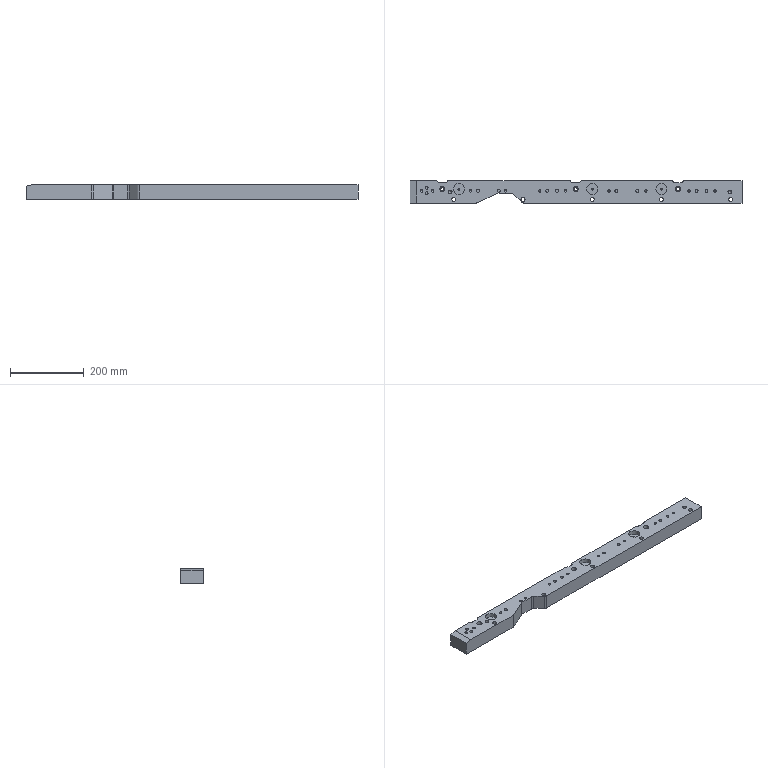Part | NX | features 22 2 | 1 solid | 112 faces | box 902 x 60 x 40 mm | volume 1958652 mm3 | cylinder 58 | plane 39 | cone 15 | commonest cylinder face diameters 6.8 x10 8.001 x10 14 x9 6 x6 11 x5 20 x4